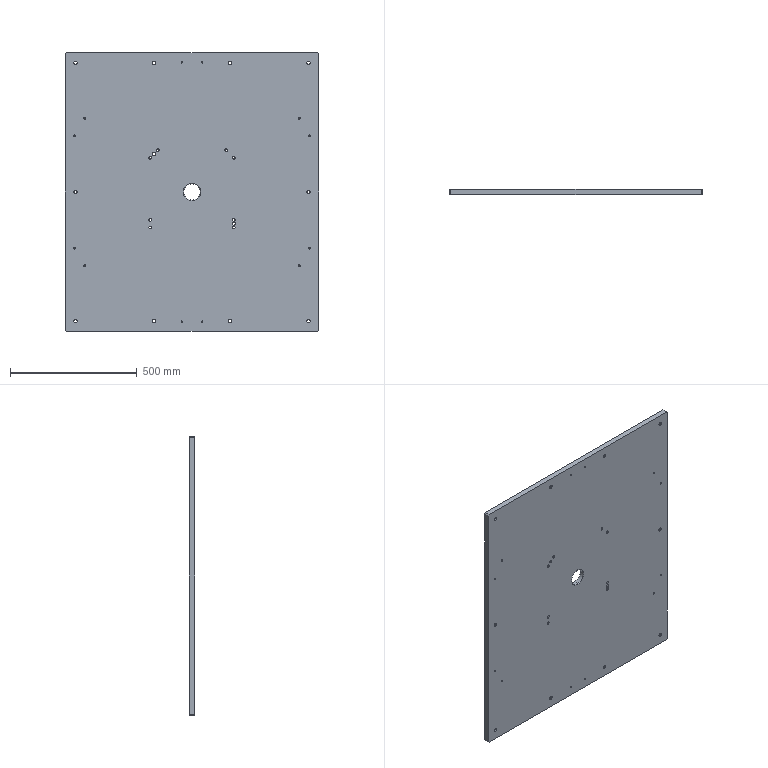Part | SolidWorks | features BaseBody 1 | 1 solid | 110 faces | box 1000 x 20 x 1100 mm | volume 21854626 mm3 | cylinder 86 | plane 20 | cone 4 | commonest cylinder face diameters 6.8 x24 13.5 x20 20 x20 10.2 x16 12 x4 65 x2